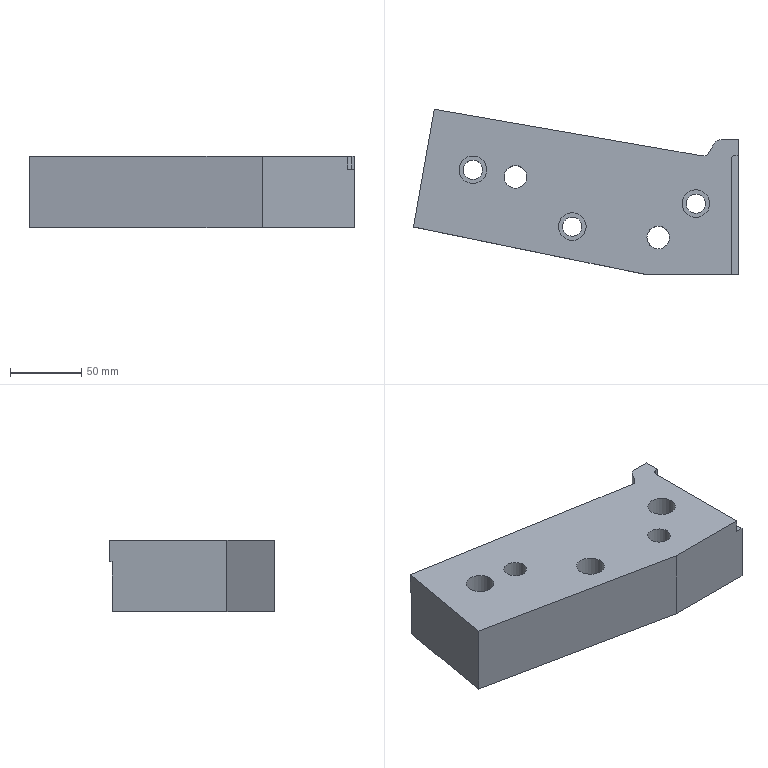Part | NX | features solid 2 | 1 solid | 29 faces | box 228.769 x 116.376 x 50 mm | volume 905067 mm3 | plane 16 | cylinder 9 | spline 4 | commonest cylinder face diameters 13.5 x3 19.5 x3 16 x2 6 x1
STEP:
#1=CARTESIAN_POINT('',(1123.262,283.786,0.));
#2=VERTEX_POINT('',#1);
#3=CARTESIAN_POINT('',(1133.012,283.786,0.));
#4=DIRECTION('',(0.,0.,-1.));
#5=DIRECTION('',(-1.,0.,0.));
#6=AXIS2_PLACEMENT_3D('',#3,#4,#5);
#7=CIRCLE('',#6,9.75);
#8=EDGE_CURVE('',#2,#2,#7,.F.);
#9=ORIENTED_EDGE('',*,*,#8,.F.);
#10=EDGE_LOOP('',(#9));
#11=FACE_BOUND('',#10,.T.);
#12=CARTESIAN_POINT('',(1053.262,323.786,0.));
#13=VERTEX_POINT('',#12);
#14=CARTESIAN_POINT('',(1063.012,323.786,0.));
#15=DIRECTION('',(0.,0.,-1.));
#16=DIRECTION('',(-1.,0.,0.));
#17=AXIS2_PLACEMENT_3D('',#14,#15,#16);
#18=CIRCLE('',#17,9.75);
#19=EDGE_CURVE('',#13,#13,#18,.F.);
#20=ORIENTED_EDGE('',*,*,#19,.F.);
#21=EDGE_LOOP('',(#20));
#22=FACE_BOUND('',#21,.T.);
#23=CARTESIAN_POINT('',(1210.25,300.,0.));
#24=VERTEX_POINT('',#23);
#25=CARTESIAN_POINT('',(1220.,300.,0.));
#26=DIRECTION('',(0.,0.,-1.));
#27=DIRECTION('',(-1.,0.,0.));
#28=AXIS2_PLACEMENT_3D('',#25,#26,#27);
#29=CIRCLE('',#28,9.75);
#30=EDGE_CURVE('',#24,#24,#29,.F.);
#31=ORIENTED_EDGE('',*,*,#30,.F.);
#32=EDGE_LOOP('',(#31));
#33=FACE_BOUND('',#32,.T.);
#34=CARTESIAN_POINT('',(1185.589,276.087,0.));
#35=VERTEX_POINT('',#34);
#36=CARTESIAN_POINT('',(1193.589,276.087,0.));
#37=DIRECTION('',(0.,0.,-1.));
#38=DIRECTION('',(-1.,0.,0.));
#39=AXIS2_PLACEMENT_3D('',#36,#37,#38);
#40=CIRCLE('',#39,8.);
#41=EDGE_CURVE('',#35,#35,#40,.F.);
#42=ORIENTED_EDGE('',*,*,#41,.F.);
#43=EDGE_LOOP('',(#42));
#44=FACE_BOUND('',#43,.T.);
#45=CARTESIAN_POINT('',(1021.231,283.553,0.));
#46=VERTEX_POINT('',#45);
#47=CARTESIAN_POINT('',(1035.834,366.376,0.));
#48=VERTEX_POINT('',#47);
#49=CARTESIAN_POINT('',(1025.414,307.279,0.));
#50=DIRECTION('',(0.1736,0.9848,0.));
#51=VECTOR('',#50,1000.);
#52=LINE('',#49,#51);
#53=EDGE_CURVE('',#46,#48,#52,.T.);
#54=ORIENTED_EDGE('',*,*,#53,.F.);
#55=CARTESIAN_POINT('',(1185.,250.,0.));
#56=VERTEX_POINT('',#55);
#57=CARTESIAN_POINT('',(1017.086,284.403,0.));
#58=DIRECTION('',(0.9797,-0.2007,0.));
#59=VECTOR('',#58,1000.);
#60=LINE('',#57,#59);
#61=EDGE_CURVE('',#46,#56,#60,.T.);
#62=ORIENTED_EDGE('',*,*,#61,.T.);
#63=CARTESIAN_POINT('',(1245.,250.,0.));
#64=VERTEX_POINT('',#63);
#65=CARTESIAN_POINT('',(1245.,250.,0.));
#66=DIRECTION('',(-1.,0.,0.));
#67=VECTOR('',#66,1000.);
#68=LINE('',#65,#67);
#69=EDGE_CURVE('',#56,#64,#68,.F.);
#70=ORIENTED_EDGE('',*,*,#69,.T.);
#71=CARTESIAN_POINT('',(1245.,331.,0.));
#72=VERTEX_POINT('',#71);
#73=CARTESIAN_POINT('',(1245.,307.899,0.));
#74=DIRECTION('',(0.,1.,0.));
#75=VECTOR('',#74,1000.);
#76=LINE('',#73,#75);
#77=EDGE_CURVE('',#64,#72,#76,.T.);
#78=ORIENTED_EDGE('',*,*,#77,.T.);
#79=CARTESIAN_POINT('',(1248.,334.,0.));
#80=VERTEX_POINT('',#79);
#81=CARTESIAN_POINT('',(1248.,331.,0.));
#82=DIRECTION('',(0.,0.,-1.));
#83=DIRECTION('',(-1.,0.,0.));
#84=AXIS2_PLACEMENT_3D('',#81,#82,#83);
#85=CIRCLE('',#84,3.);
#86=EDGE_CURVE('',#72,#80,#85,.T.);
#87=ORIENTED_EDGE('',*,*,#86,.T.);
#88=CARTESIAN_POINT('',(1250.,334.,0.));
#89=VERTEX_POINT('',#88);
#90=CARTESIAN_POINT('',(1021.9,334.,0.));
#91=DIRECTION('',(1.,0.,0.));
#92=VECTOR('',#91,1000.);
#93=LINE('',#90,#92);
#94=EDGE_CURVE('',#89,#80,#93,.F.);
#95=ORIENTED_EDGE('',*,*,#94,.F.);
#96=CARTESIAN_POINT('',(1250.,345.,0.));
#97=VERTEX_POINT('',#96);
#98=CARTESIAN_POINT('',(1250.,340.,0.));
#99=DIRECTION('',(0.,-1.,0.));
#100=VECTOR('',#99,1000.);
#101=LINE('',#98,#100);
#102=EDGE_CURVE('',#97,#89,#101,.T.);
#103=ORIENTED_EDGE('',*,*,#102,.F.);
#104=CARTESIAN_POINT('',(1237.889,345.,0.));
#105=VERTEX_POINT('',#104);
#106=CARTESIAN_POINT('',(1021.9,345.,0.));
#107=DIRECTION('',(-1.,0.,0.));
#108=VECTOR('',#107,1000.);
#109=LINE('',#106,#108);
#110=EDGE_CURVE('',#97,#105,#109,.T.);
#111=ORIENTED_EDGE('',*,*,#110,.T.);
#112=CARTESIAN_POINT('',(1231.463,339.803,0.));
#113=VERTEX_POINT('',#112);
#114=CARTESIAN_POINT('',(1231.463,339.803,0.));
#115=CARTESIAN_POINT('',(1232.171,341.078,0.));
#116=CARTESIAN_POINT('',(1233.286,342.988,0.));
#117=CARTESIAN_POINT('',(1235.696,344.739,0.));
#118=CARTESIAN_POINT('',(1237.155,345.,0.));
#119=CARTESIAN_POINT('',(1237.889,345.,0.));
#120=B_SPLINE_CURVE_WITH_KNOTS('',3,(#114,#115,#116,#117,#118,#119),.UNSPECIFIED.,.F.,.F.,(4,1,1,4),(0.05738,0.06181,0.06402,0.06624),.UNSPECIFIED.);
#121=EDGE_CURVE('',#113,#105,#120,.T.);
#122=ORIENTED_EDGE('',*,*,#121,.F.);
#123=CARTESIAN_POINT('',(1224.486,333.568,0.));
#124=VERTEX_POINT('',#123);
#125=CARTESIAN_POINT('',(1224.486,333.568,0.));
#126=CARTESIAN_POINT('',(1231.05,332.426,0.));
#127=CARTESIAN_POINT('',(1230.692,345.,0.));
#128=CARTESIAN_POINT('',(1237.854,345.,0.));
#129=B_SPLINE_CURVE_WITH_KNOTS('',3,(#125,#126,#127,#128),.UNSPECIFIED.,.F.,.F.,(4,4),(0.,1.),.PIECEWISE_BEZIER_KNOTS.);
#130=EDGE_CURVE('',#124,#113,#129,.T.);
#131=ORIENTED_EDGE('',*,*,#130,.F.);
#132=CARTESIAN_POINT('',(1187.5,340.,0.));
#133=VERTEX_POINT('',#132);
#134=CARTESIAN_POINT('',(1228.,332.956,0.));
#135=DIRECTION('',(-0.9852,0.1713,0.));
#136=VECTOR('',#135,1000.);
#137=LINE('',#134,#136);
#138=EDGE_CURVE('',#124,#133,#137,.T.);
#139=ORIENTED_EDGE('',*,*,#138,.T.);
#140=CARTESIAN_POINT('',(1323.576,316.335,0.));
#141=CARTESIAN_POINT('',(1303.952,319.748,0.));
#142=CARTESIAN_POINT('',(1284.328,323.16,0.));
#143=CARTESIAN_POINT('',(1264.704,326.573,0.));
#144=CARTESIAN_POINT('',(1233.889,331.932,0.));
#145=CARTESIAN_POINT('',(1172.258,342.651,0.));
#146=CARTESIAN_POINT('',(1095.22,356.049,0.));
#147=CARTESIAN_POINT('',(1033.589,366.767,0.));
#148=CARTESIAN_POINT('',(987.365,374.804,0.));
#149=CARTESIAN_POINT('',(948.847,381.509,0.));
#150=CARTESIAN_POINT('',(923.808,385.853,0.));
#151=CARTESIAN_POINT('',(914.109,387.486,0.));
#152=CARTESIAN_POINT('',(912.091,387.827,0.));
#153=CARTESIAN_POINT('',(911.971,387.848,0.));
#154=CARTESIAN_POINT('',(911.79,387.876,0.));
#155=CARTESIAN_POINT('',(911.394,387.917,0.));
#156=CARTESIAN_POINT('',(910.546,388.022,0.));
#157=CARTESIAN_POINT('',(908.847,388.221,0.));
#158=CARTESIAN_POINT('',(906.42,388.511,0.));
#159=CARTESIAN_POINT('',(903.994,388.799,0.));
#160=CARTESIAN_POINT('',(902.295,389.001,0.));
#161=CARTESIAN_POINT('',(901.446,389.101,0.));
#162=CARTESIAN_POINT('',(901.052,389.148,0.));
#163=CARTESIAN_POINT('',(900.87,389.17,0.));
#164=CARTESIAN_POINT('',(900.748,389.184,0.));
#165=CARTESIAN_POINT('',(899.68,389.239,0.));
#166=CARTESIAN_POINT('',(897.973,389.35,0.));
#167=CARTESIAN_POINT('',(896.023,389.486,0.));
#168=CARTESIAN_POINT('',(894.456,389.561,0.));
#169=CARTESIAN_POINT('',(892.989,389.903,0.));
#170=CARTESIAN_POINT('',(891.495,390.907,0.));
#171=CARTESIAN_POINT('',(890.458,392.378,0.));
#172=CARTESIAN_POINT('',(890.077,393.863,0.));
#173=CARTESIAN_POINT('',(889.825,397.101,0.));
#174=CARTESIAN_POINT('',(889.362,402.393,0.));
#175=CARTESIAN_POINT('',(888.928,407.354,0.));
#176=CARTESIAN_POINT('',(888.696,410.,0.));
#177=CARTESIAN_POINT('',(886.96,429.843,0.));
#178=CARTESIAN_POINT('',(885.224,449.685,0.));
#179=CARTESIAN_POINT('',(883.488,469.528,0.));
#180=B_SPLINE_CURVE_WITH_KNOTS('',3,(#140,#141,#142,#143,#144,#145,#146,#147,#148,#149,#150,#151,#152,#153,#154,#155,#156,#157,#158,#159,#160,#161,#162,#163,#164,#165,#166,#167,#168,#169,#170,#171,#172,#173,#174,#175,#176,#177,#178,#179),.UNSPECIFIED.,.F.,.F.,(4,3,1,1,1,1,1,1,1,1,1,1,1,1,1,1,1,1,1,1,1,1,1,1,1,1,1,1,1,1,1,1,3,4),(-0.15,0.,0.2355,0.4711,0.5889,0.7066,0.8244,0.8833,0.898,0.8985,0.8987,0.8989,0.8999,0.9017,0.9054,0.9127,0.9201,0.9238,0.9256,0.9265,0.9268,0.927,0.9275,0.9348,0.9399,0.9422,0.9466,0.9511,0.9555,0.96,0.9625,0.98,1.,1.15),.UNSPECIFIED.);
#181=EDGE_CURVE('',#133,#48,#180,.T.);
#182=ORIENTED_EDGE('',*,*,#181,.T.);
#183=EDGE_LOOP('',(#54,#62,#70,#78,#87,#95,#103,#111,#122,#131,#139,#182));
#184=FACE_BOUND('',#183,.T.);
#185=CARTESIAN_POINT('',(1085.012,318.786,0.));
#186=VERTEX_POINT('',#185);
#187=CARTESIAN_POINT('',(1093.012,318.786,0.));
#188=DIRECTION('',(0.,0.,-1.));
#189=DIRECTION('',(-1.,0.,0.));
#190=AXIS2_PLACEMENT_3D('',#187,#188,#189);
#191=CIRCLE('',#190,8.);
#192=EDGE_CURVE('',#186,#186,#191,.F.);
#193=ORIENTED_EDGE('',*,*,#192,.F.);
#194=EDGE_LOOP('',(#193));
#195=FACE_BOUND('',#194,.T.);
#196=CARTESIAN_POINT('',(1021.9,307.899,0.));
#197=DIRECTION('',(0.,0.,-1.));
#198=DIRECTION('',(1.,0.,0.));
#199=AXIS2_PLACEMENT_3D('',#196,#197,#198);
#200=PLANE('',#199);
#201=ADVANCED_FACE('',(#11,#22,#33,#44,#184,#195),#200,.F.);
#202=CARTESIAN_POINT('',(1126.262,283.786,-50.));
#203=VERTEX_POINT('',#202);
#204=CARTESIAN_POINT('',(1133.012,283.786,-50.));
#205=DIRECTION('',(0.,0.,-1.));
#206=DIRECTION('',(-1.,0.,0.));
#207=AXIS2_PLACEMENT_3D('',#204,#205,#206);
#208=CIRCLE('',#207,6.75);
#209=EDGE_CURVE('',#203,#203,#208,.F.);
#210=ORIENTED_EDGE('',*,*,#209,.T.);
#211=EDGE_LOOP('',(#210));
#212=FACE_BOUND('',#211,.T.);
#213=CARTESIAN_POINT('',(1056.262,323.786,-50.));
#214=VERTEX_POINT('',#213);
#215=CARTESIAN_POINT('',(1063.012,323.786,-50.));
#216=DIRECTION('',(0.,0.,-1.));
#217=DIRECTION('',(-1.,0.,0.));
#218=AXIS2_PLACEMENT_3D('',#215,#216,#217);
#219=CIRCLE('',#218,6.75);
#220=EDGE_CURVE('',#214,#214,#219,.F.);
#221=ORIENTED_EDGE('',*,*,#220,.T.);
#222=EDGE_LOOP('',(#221));
#223=FACE_BOUND('',#222,.T.);
#224=CARTESIAN_POINT('',(1213.25,300.,-50.));
#225=VERTEX_POINT('',#224);
#226=CARTESIAN_POINT('',(1220.,300.,-50.));
#227=DIRECTION('',(0.,0.,-1.));
#228=DIRECTION('',(-1.,0.,0.));
#229=AXIS2_PLACEMENT_3D('',#226,#227,#228);
#230=CIRCLE('',#229,6.75);
#231=EDGE_CURVE('',#225,#225,#230,.F.);
#232=ORIENTED_EDGE('',*,*,#231,.T.);
#233=EDGE_LOOP('',(#232));
#234=FACE_BOUND('',#233,.T.);
#235=CARTESIAN_POINT('',(1185.589,276.087,-50.));
#236=VERTEX_POINT('',#235);
#237=CARTESIAN_POINT('',(1193.589,276.087,-50.));
#238=DIRECTION('',(0.,0.,-1.));
#239=DIRECTION('',(-1.,0.,0.));
#240=AXIS2_PLACEMENT_3D('',#237,#238,#239);
#241=CIRCLE('',#240,8.);
#242=EDGE_CURVE('',#236,#236,#241,.F.);
#243=ORIENTED_EDGE('',*,*,#242,.T.);
#244=EDGE_LOOP('',(#243));
#245=FACE_BOUND('',#244,.T.);
#246=CARTESIAN_POINT('',(1021.231,283.553,-50.));
#247=VERTEX_POINT('',#246);
#248=CARTESIAN_POINT('',(1185.,250.,-50.));
#249=VERTEX_POINT('',#248);
#250=CARTESIAN_POINT('',(1017.086,284.403,-50.));
#251=DIRECTION('',(0.9797,-0.2007,0.));
#252=VECTOR('',#251,1000.);
#253=LINE('',#250,#252);
#254=EDGE_CURVE('',#247,#249,#253,.T.);
#255=ORIENTED_EDGE('',*,*,#254,.F.);
#256=CARTESIAN_POINT('',(1035.487,364.407,-50.));
#257=VERTEX_POINT('',#256);
#258=CARTESIAN_POINT('',(1025.414,307.279,-50.));
#259=DIRECTION('',(0.1736,0.9848,0.));
#260=VECTOR('',#259,1000.);
#261=LINE('',#258,#260);
#262=EDGE_CURVE('',#247,#257,#261,.T.);
#263=ORIENTED_EDGE('',*,*,#262,.T.);
#264=CARTESIAN_POINT('',(1224.144,331.597,-50.));
#265=VERTEX_POINT('',#264);
#266=CARTESIAN_POINT('',(1035.487,364.408,-50.));
#267=CARTESIAN_POINT('',(1098.372,353.464,-50.));
#268=CARTESIAN_POINT('',(1161.256,342.523,-50.));
#269=CARTESIAN_POINT('',(1224.143,331.595,-50.));
#270=B_SPLINE_CURVE_WITH_KNOTS('',3,(#266,#267,#268,#269),.UNSPECIFIED.,.F.,.F.,(4,4),(0.4726,0.9521),.UNSPECIFIED.);
#271=EDGE_CURVE('',#265,#257,#270,.F.);
#272=ORIENTED_EDGE('',*,*,#271,.F.);
#273=CARTESIAN_POINT('',(1232.756,337.998,-50.));
#274=VERTEX_POINT('',#273);
#275=CARTESIAN_POINT('',(1224.143,331.597,-50.));
#276=CARTESIAN_POINT('',(1225.228,331.409,-50.));
#277=CARTESIAN_POINT('',(1226.743,331.5,-50.));
#278=CARTESIAN_POINT('',(1228.346,332.296,-50.));
#279=CARTESIAN_POINT('',(1229.18,332.908,-50.));
#280=CARTESIAN_POINT('',(1229.861,333.556,-50.));
#281=CARTESIAN_POINT('',(1230.2,333.942,-50.));
#282=CARTESIAN_POINT('',(1230.629,334.473,-50.));
#283=CARTESIAN_POINT('',(1230.974,334.958,-50.));
#284=CARTESIAN_POINT('',(1231.239,335.355,-50.));
#285=CARTESIAN_POINT('',(1231.48,335.737,-50.));
#286=CARTESIAN_POINT('',(1231.56,335.871,-50.));
#287=CARTESIAN_POINT('',(1231.745,336.182,-50.));
#288=CARTESIAN_POINT('',(1232.087,336.777,-50.));
#289=CARTESIAN_POINT('',(1232.468,337.468,-50.));
#290=CARTESIAN_POINT('',(1232.756,337.998,-50.));
#291=B_SPLINE_CURVE_WITH_KNOTS('',3,(#275,#276,#277,#278,#279,#280,#281,#282,#283,#284,#285,#286,#287,#288,#289,#290),.UNSPECIFIED.,.F.,.F.,(4,1,1,1,1,1,1,1,1,1,1,1,1,4),(0.,0.25,0.375,0.4375,0.5,0.5625,0.625,0.6875,0.7188,0.75,0.7812,0.8125,0.875,1.),.UNSPECIFIED.);
#292=EDGE_CURVE('',#265,#274,#291,.T.);
#293=ORIENTED_EDGE('',*,*,#292,.T.);
#294=CARTESIAN_POINT('',(1237.854,343.,-50.));
#295=VERTEX_POINT('',#294);
#296=CARTESIAN_POINT('',(1232.755,337.999,-50.));
#297=CARTESIAN_POINT('',(1233.177,338.771,-50.));
#298=CARTESIAN_POINT('',(1233.575,339.487,-50.));
#299=CARTESIAN_POINT('',(1233.966,340.122,-50.));
#300=CARTESIAN_POINT('',(1234.076,340.296,-50.));
#301=CARTESIAN_POINT('',(1234.264,340.582,-50.));
#302=CARTESIAN_POINT('',(1234.523,340.953,-50.));
#303=CARTESIAN_POINT('',(1234.918,341.464,-50.));
#304=CARTESIAN_POINT('',(1235.316,341.895,-50.));
#305=CARTESIAN_POINT('',(1235.691,342.232,-50.));
#306=CARTESIAN_POINT('',(1236.515,342.818,-50.));
#307=CARTESIAN_POINT('',(1237.221,343.,-50.));
#308=CARTESIAN_POINT('',(1237.854,343.,-50.));
#309=B_SPLINE_CURVE_WITH_KNOTS('',3,(#296,#297,#298,#299,#300,#301,#302,#303,#304,#305,#306,#307,#308),.UNSPECIFIED.,.F.,.F.,(4,1,1,1,1,1,1,1,1,1,4),(0.613,0.7098,0.734,0.7461,0.7582,0.7823,0.8065,0.8549,0.8791,0.9033,1.),.UNSPECIFIED.);
#310=EDGE_CURVE('',#274,#295,#309,.T.);
#311=ORIENTED_EDGE('',*,*,#310,.T.);
#312=CARTESIAN_POINT('',(1250.,343.,-50.));
#313=VERTEX_POINT('',#312);
#314=CARTESIAN_POINT('',(1021.9,343.,-50.));
#315=DIRECTION('',(-1.,0.,0.));
#316=VECTOR('',#315,1000.);
#317=LINE('',#314,#316);
#318=EDGE_CURVE('',#313,#295,#317,.T.);
#319=ORIENTED_EDGE('',*,*,#318,.F.);
#320=CARTESIAN_POINT('',(1250.,250.,-50.));
#321=VERTEX_POINT('',#320);
#322=CARTESIAN_POINT('',(1250.,307.899,-50.));
#323=DIRECTION('',(0.,1.,0.));
#324=VECTOR('',#323,1000.);
#325=LINE('',#322,#324);
#326=EDGE_CURVE('',#321,#313,#325,.T.);
#327=ORIENTED_EDGE('',*,*,#326,.F.);
#328=CARTESIAN_POINT('',(1245.,250.,-50.));
#329=DIRECTION('',(-1.,0.,0.));
#330=VECTOR('',#329,1000.);
#331=LINE('',#328,#330);
#332=EDGE_CURVE('',#321,#249,#331,.T.);
#333=ORIENTED_EDGE('',*,*,#332,.T.);
#334=EDGE_LOOP('',(#255,#263,#272,#293,#311,#319,#327,#333));
#335=FACE_BOUND('',#334,.T.);
#336=CARTESIAN_POINT('',(1085.012,318.786,-50.));
#337=VERTEX_POINT('',#336);
#338=CARTESIAN_POINT('',(1093.012,318.786,-50.));
#339=DIRECTION('',(0.,0.,-1.));
#340=DIRECTION('',(-1.,0.,0.));
#341=AXIS2_PLACEMENT_3D('',#338,#339,#340);
#342=CIRCLE('',#341,8.);
#343=EDGE_CURVE('',#337,#337,#342,.F.);
#344=ORIENTED_EDGE('',*,*,#343,.T.);
#345=EDGE_LOOP('',(#344));
#346=FACE_BOUND('',#345,.T.);
#347=CARTESIAN_POINT('',(1021.9,307.899,-50.));
#348=DIRECTION('',(0.,0.,-1.));
#349=DIRECTION('',(1.,0.,0.));
#350=AXIS2_PLACEMENT_3D('',#347,#348,#349);
#351=PLANE('',#350);
#352=ADVANCED_FACE('',(#212,#223,#234,#245,#335,#346),#351,.T.);
#353=CARTESIAN_POINT('',(1035.487,364.406,-15.));
#354=VERTEX_POINT('',#353);
#355=CARTESIAN_POINT('',(1035.487,364.406,-32.5));
#356=DIRECTION('',(0.,0.,1.));
#357=VECTOR('',#356,1000.);
#358=LINE('',#355,#357);
#359=EDGE_CURVE('',#354,#257,#358,.F.);
#360=ORIENTED_EDGE('',*,*,#359,.F.);
#361=CARTESIAN_POINT('',(1224.143,331.597,-15.));
#362=VERTEX_POINT('',#361);
#363=CARTESIAN_POINT('',(1035.487,364.406,-15.));
#364=CARTESIAN_POINT('',(1098.373,353.471,-15.));
#365=CARTESIAN_POINT('',(1161.258,342.534,-15.));
#366=CARTESIAN_POINT('',(1224.143,331.597,-15.));
#367=B_SPLINE_CURVE_WITH_KNOTS('',3,(#363,#364,#365,#366),.UNSPECIFIED.,.F.,.F.,(4,4),(0.8083,0.9998),.UNSPECIFIED.);
#368=EDGE_CURVE('',#362,#354,#367,.F.);
#369=ORIENTED_EDGE('',*,*,#368,.F.);
#370=CARTESIAN_POINT('',(1224.143,331.597,-15.));
#371=DIRECTION('',(0.,0.,-1.));
#372=VECTOR('',#371,1000.);
#373=LINE('',#370,#372);
#374=EDGE_CURVE('',#362,#265,#373,.T.);
#375=ORIENTED_EDGE('',*,*,#374,.T.);
#376=ORIENTED_EDGE('',*,*,#271,.T.);
#377=EDGE_LOOP('',(#360,#369,#375,#376));
#378=FACE_BOUND('',#377,.T.);
#379=CARTESIAN_POINT('',(1225.276,331.4,-50.));
#380=CARTESIAN_POINT('',(1225.276,331.4,-15.));
#381=CARTESIAN_POINT('',(1162.013,342.402,-50.));
#382=CARTESIAN_POINT('',(1162.013,342.402,-15.));
#383=CARTESIAN_POINT('',(1098.75,353.405,-50.));
#384=CARTESIAN_POINT('',(1098.75,353.405,-15.));
#385=CARTESIAN_POINT('',(1035.487,364.406,-50.));
#386=CARTESIAN_POINT('',(1035.487,364.406,-15.));
#387=B_SPLINE_SURFACE_WITH_KNOTS('',3,1,((#379,#380),(#381,#382),(#383,#384),(#385,#386)),.SURF_OF_LINEAR_EXTRUSION.,.F.,.F.,.F.,(4,4),(2,2),(0.09649,0.5817),(0.,1.),.PIECEWISE_BEZIER_KNOTS.);
#388=ADVANCED_FACE('',(#378),#387,.T.);
#389=CARTESIAN_POINT('',(1035.834,366.376,-15.));
#390=VERTEX_POINT('',#389);
#391=CARTESIAN_POINT('',(1035.834,366.376,-7.5));
#392=DIRECTION('',(0.,0.,1.));
#393=VECTOR('',#392,1000.);
#394=LINE('',#391,#393);
#395=EDGE_CURVE('',#48,#390,#394,.F.);
#396=ORIENTED_EDGE('',*,*,#395,.F.);
#397=ORIENTED_EDGE('',*,*,#181,.F.);
#398=CARTESIAN_POINT('',(1187.5,340.,-15.));
#399=VERTEX_POINT('',#398);
#400=CARTESIAN_POINT('',(1187.5,340.,0.));
#401=DIRECTION('',(0.,0.,-1.));
#402=VECTOR('',#401,1000.);
#403=LINE('',#400,#402);
#404=EDGE_CURVE('',#399,#133,#403,.F.);
#405=ORIENTED_EDGE('',*,*,#404,.F.);
#406=CARTESIAN_POINT('',(1045.24,364.741,-15.));
#407=VERTEX_POINT('',#406);
#408=CARTESIAN_POINT('',(1187.5,340.,-15.));
#409=CARTESIAN_POINT('',(1140.08,348.247,-15.));
#410=CARTESIAN_POINT('',(1092.66,356.494,-15.));
#411=CARTESIAN_POINT('',(1045.24,364.741,-15.));
#412=B_SPLINE_CURVE_WITH_KNOTS('',3,(#408,#409,#410,#411),.UNSPECIFIED.,.F.,.F.,(4,4),(0.05836,0.2028),.UNSPECIFIED.);
#413=EDGE_CURVE('',#399,#407,#412,.T.);
#414=ORIENTED_EDGE('',*,*,#413,.T.);
#415=CARTESIAN_POINT('',(1035.834,366.376,-15.));
#416=CARTESIAN_POINT('',(1038.848,365.852,-15.));
#417=CARTESIAN_POINT('',(1041.983,365.307,-15.));
#418=CARTESIAN_POINT('',(1045.24,364.741,-15.));
#419=B_SPLINE_CURVE_WITH_KNOTS('',3,(#415,#416,#417,#418),.UNSPECIFIED.,.F.,.F.,(4,4),(0.9049,1.),.UNSPECIFIED.);
#420=EDGE_CURVE('',#407,#390,#419,.F.);
#421=ORIENTED_EDGE('',*,*,#420,.T.);
#422=EDGE_LOOP('',(#396,#397,#405,#414,#421));
#423=FACE_BOUND('',#422,.T.);
#424=CARTESIAN_POINT('',(1187.5,340.,-15.));
#425=CARTESIAN_POINT('',(1187.5,340.,0.));
#426=CARTESIAN_POINT('',(1136.945,348.792,-15.));
#427=CARTESIAN_POINT('',(1136.945,348.792,0.));
#428=CARTESIAN_POINT('',(1086.39,357.585,-15.));
#429=CARTESIAN_POINT('',(1086.39,357.585,0.));
#430=CARTESIAN_POINT('',(1035.834,366.376,-15.));
#431=CARTESIAN_POINT('',(1035.834,366.376,0.));
#432=B_SPLINE_SURFACE_WITH_KNOTS('',3,1,((#424,#425),(#426,#427),(#428,#429),(#430,#431)),.SURF_OF_LINEAR_EXTRUSION.,.F.,.F.,.F.,(4,4),(2,2),(0.1967,0.5831),(0.,1.),.PIECEWISE_BEZIER_KNOTS.);
#433=ADVANCED_FACE('',(#423),#432,.T.);
#434=CARTESIAN_POINT('',(1022.389,290.122,-15.));
#435=DIRECTION('',(0.1736,0.9848,0.));
#436=VECTOR('',#435,1000.);
#437=LINE('',#434,#436);
#438=EDGE_CURVE('',#390,#354,#437,.F.);
#439=ORIENTED_EDGE('',*,*,#438,.F.);
#440=ORIENTED_EDGE('',*,*,#420,.F.);
#441=ORIENTED_EDGE('',*,*,#413,.F.);
#442=CARTESIAN_POINT('',(1224.486,333.568,-15.));
#443=VERTEX_POINT('',#442);
#444=CARTESIAN_POINT('',(1258.358,327.677,-15.));
#445=DIRECTION('',(0.9852,-0.1713,0.));
#446=VECTOR('',#445,1000.);
#447=LINE('',#444,#446);
#448=EDGE_CURVE('',#443,#399,#447,.F.);
#449=ORIENTED_EDGE('',*,*,#448,.F.);
#450=CARTESIAN_POINT('',(1237.854,345.,-15.));
#451=VERTEX_POINT('',#450);
#452=CARTESIAN_POINT('',(1224.486,333.568,-15.));
#453=CARTESIAN_POINT('',(1231.05,332.426,-15.));
#454=CARTESIAN_POINT('',(1230.692,345.,-15.));
#455=CARTESIAN_POINT('',(1237.854,345.,-15.));
#456=B_SPLINE_CURVE_WITH_KNOTS('',3,(#452,#453,#454,#455),.UNSPECIFIED.,.F.,.F.,(4,4),(0.,1.),.PIECEWISE_BEZIER_KNOTS.);
#457=EDGE_CURVE('',#443,#451,#456,.T.);
#458=ORIENTED_EDGE('',*,*,#457,.T.);
#459=CARTESIAN_POINT('',(1250.,345.,-15.));
#460=VERTEX_POINT('',#459);
#461=CARTESIAN_POINT('',(1250.,345.,-15.));
#462=DIRECTION('',(-1.,0.,0.));
#463=VECTOR('',#462,1000.);
#464=LINE('',#461,#463);
#465=EDGE_CURVE('',#460,#451,#464,.T.);
#466=ORIENTED_EDGE('',*,*,#465,.F.);
#467=CARTESIAN_POINT('',(1250.,343.,-15.));
#468=VERTEX_POINT('',#467);
#469=CARTESIAN_POINT('',(1250.,390.,-15.));
#470=DIRECTION('',(0.,1.,0.));
#471=VECTOR('',#470,1000.);
#472=LINE('',#469,#471);
#473=EDGE_CURVE('',#460,#468,#472,.F.);
#474=ORIENTED_EDGE('',*,*,#473,.T.);
#475=CARTESIAN_POINT('',(1237.854,343.,-15.));
#476=VERTEX_POINT('',#475);
#477=CARTESIAN_POINT('',(1250.,343.,-15.));
#478=DIRECTION('',(-1.,0.,0.));
#479=VECTOR('',#478,1000.);
#480=LINE('',#477,#479);
#481=EDGE_CURVE('',#468,#476,#480,.T.);
#482=ORIENTED_EDGE('',*,*,#481,.T.);
#483=CARTESIAN_POINT('',(1233.89,340.,-15.));
#484=VERTEX_POINT('',#483);
#485=CARTESIAN_POINT('',(1233.89,340.,-15.));
#486=CARTESIAN_POINT('',(1234.534,341.043,-15.));
#487=CARTESIAN_POINT('',(1235.689,342.507,-15.));
#488=CARTESIAN_POINT('',(1237.072,343.,-15.));
#489=CARTESIAN_POINT('',(1237.854,343.,-15.));
#490=B_SPLINE_CURVE_WITH_KNOTS('',3,(#485,#486,#487,#488,#489),.UNSPECIFIED.,.F.,.F.,(4,1,4),(0.,0.5,1.),.UNSPECIFIED.);
#491=EDGE_CURVE('',#484,#476,#490,.T.);
#492=ORIENTED_EDGE('',*,*,#491,.F.);
#493=CARTESIAN_POINT('',(1232.756,337.998,-15.));
#494=VERTEX_POINT('',#493);
#495=CARTESIAN_POINT('',(1233.89,340.,-15.));
#496=CARTESIAN_POINT('',(1233.512,339.333,-15.));
#497=CARTESIAN_POINT('',(1233.134,338.666,-15.));
#498=CARTESIAN_POINT('',(1232.756,337.998,-15.));
#499=B_SPLINE_CURVE_WITH_KNOTS('',3,(#495,#496,#497,#498),.UNSPECIFIED.,.F.,.F.,(4,4),(0.,1.),.UNSPECIFIED.);
#500=EDGE_CURVE('',#494,#484,#499,.F.);
#501=ORIENTED_EDGE('',*,*,#500,.F.);
#502=CARTESIAN_POINT('',(1224.143,331.597,-15.));
#503=CARTESIAN_POINT('',(1225.228,331.409,-15.));
#504=CARTESIAN_POINT('',(1226.744,331.502,-15.));
#505=CARTESIAN_POINT('',(1228.342,332.293,-15.));
#506=CARTESIAN_POINT('',(1229.183,332.912,-15.));
#507=CARTESIAN_POINT('',(1229.842,333.536,-15.));
#508=CARTESIAN_POINT('',(1230.19,333.929,-15.));
#509=CARTESIAN_POINT('',(1230.626,334.469,-15.));
#510=CARTESIAN_POINT('',(1231.022,335.02,-15.));
#511=CARTESIAN_POINT('',(1231.411,335.625,-15.));
#512=CARTESIAN_POINT('',(1231.549,335.853,-15.));
#513=CARTESIAN_POINT('',(1231.738,336.169,-15.));
#514=CARTESIAN_POINT('',(1232.088,336.777,-15.));
#515=CARTESIAN_POINT('',(1232.494,337.517,-15.));
#516=CARTESIAN_POINT('',(1232.756,337.998,-15.));
#517=B_SPLINE_CURVE_WITH_KNOTS('',3,(#502,#503,#504,#505,#506,#507,#508,#509,#510,#511,#512,#513,#514,#515,#516),.UNSPECIFIED.,.F.,.F.,(4,1,1,1,1,1,1,1,1,1,1,1,4),(0.,0.126,0.189,0.2206,0.2521,0.2836,0.3151,0.3466,0.3781,0.3939,0.4096,0.4411,0.5041),.UNSPECIFIED.);
#518=EDGE_CURVE('',#362,#494,#517,.T.);
#519=ORIENTED_EDGE('',*,*,#518,.F.);
#520=ORIENTED_EDGE('',*,*,#368,.T.);
#521=EDGE_LOOP('',(#439,#440,#441,#449,#458,#466,#474,#482,#492,#501,#519,#520));
#522=FACE_BOUND('',#521,.T.);
#523=CARTESIAN_POINT('',(1245.,250.87,-15.));
#524=DIRECTION('',(0.,0.,-1.));
#525=DIRECTION('',(0.,1.,0.));
#526=AXIS2_PLACEMENT_3D('',#523,#524,#525);
#527=PLANE('',#526);
#528=ADVANCED_FACE('',(#522),#527,.T.);
#529=CARTESIAN_POINT('',(1021.231,283.553,-50.));
#530=DIRECTION('',(0.,0.,1.));
#531=VECTOR('',#530,1000.);
#532=LINE('',#529,#531);
#533=EDGE_CURVE('',#247,#46,#532,.T.);
#534=ORIENTED_EDGE('',*,*,#533,.F.);
#535=ORIENTED_EDGE('',*,*,#254,.T.);
#536=CARTESIAN_POINT('',(1185.,250.,0.));
#537=DIRECTION('',(0.,0.,-1.));
#538=VECTOR('',#537,1000.);
#539=LINE('',#536,#538);
#540=EDGE_CURVE('',#56,#249,#539,.T.);
#541=ORIENTED_EDGE('',*,*,#540,.F.);
#542=ORIENTED_EDGE('',*,*,#61,.F.);
#543=EDGE_LOOP('',(#534,#535,#541,#542));
#544=FACE_BOUND('',#543,.T.);
#545=CARTESIAN_POINT('',(1185.,250.,-50.));
#546=DIRECTION('',(0.2007,0.9797,0.));
#547=DIRECTION('',(-0.9797,0.2007,0.));
#548=AXIS2_PLACEMENT_3D('',#545,#546,#547);
#549=PLANE('',#548);
#550=ADVANCED_FACE('',(#544),#549,.F.);
#551=ORIENTED_EDGE('',*,*,#102,.T.);
#552=CARTESIAN_POINT('',(1250.,334.,-9.));
#553=VERTEX_POINT('',#552);
#554=CARTESIAN_POINT('',(1250.,334.,-50.));
#555=DIRECTION('',(0.,0.,-1.));
#556=VECTOR('',#555,1000.);
#557=LINE('',#554,#556);
#558=EDGE_CURVE('',#553,#89,#557,.F.);
#559=ORIENTED_EDGE('',*,*,#558,.F.);
#560=CARTESIAN_POINT('',(1250.,250.,-9.));
#561=VERTEX_POINT('',#560);
#562=CARTESIAN_POINT('',(1250.,390.,-9.));
#563=DIRECTION('',(0.,-1.,0.));
#564=VECTOR('',#563,1000.);
#565=LINE('',#562,#564);
#566=EDGE_CURVE('',#561,#553,#565,.F.);
#567=ORIENTED_EDGE('',*,*,#566,.F.);
#568=CARTESIAN_POINT('',(1250.,250.,0.));
#569=DIRECTION('',(0.,0.,1.));
#570=VECTOR('',#569,1000.);
#571=LINE('',#568,#570);
#572=EDGE_CURVE('',#321,#561,#571,.T.);
#573=ORIENTED_EDGE('',*,*,#572,.F.);
#574=ORIENTED_EDGE('',*,*,#326,.T.);
#575=CARTESIAN_POINT('',(1250.,343.,-50.));
#576=DIRECTION('',(0.,0.,1.));
#577=VECTOR('',#576,1000.);
#578=LINE('',#575,#577);
#579=EDGE_CURVE('',#468,#313,#578,.F.);
#580=ORIENTED_EDGE('',*,*,#579,.F.);
#581=ORIENTED_EDGE('',*,*,#473,.F.);
#582=CARTESIAN_POINT('',(1250.,345.,-50.));
#583=DIRECTION('',(0.,0.,1.));
#584=VECTOR('',#583,1000.);
#585=LINE('',#582,#584);
#586=EDGE_CURVE('',#97,#460,#585,.F.);
#587=ORIENTED_EDGE('',*,*,#586,.F.);
#588=EDGE_LOOP('',(#551,#559,#567,#573,#574,#580,#581,#587));
#589=FACE_BOUND('',#588,.T.);
#590=CARTESIAN_POINT('',(1250.,390.,-50.));
#591=DIRECTION('',(-1.,0.,0.));
#592=DIRECTION('',(0.,0.,1.));
#593=AXIS2_PLACEMENT_3D('',#590,#591,#592);
#594=PLANE('',#593);
#595=ADVANCED_FACE('',(#589),#594,.F.);
#596=CARTESIAN_POINT('',(1245.,250.,-9.));
#597=VERTEX_POINT('',#596);
#598=CARTESIAN_POINT('',(1185.,250.,-9.));
#599=DIRECTION('',(-1.,0.,0.));
#600=VECTOR('',#599,1000.);
#601=LINE('',#598,#600);
#602=EDGE_CURVE('',#597,#561,#601,.F.);
#603=ORIENTED_EDGE('',*,*,#602,.F.);
#604=CARTESIAN_POINT('',(1245.,250.,0.));
#605=DIRECTION('',(0.,0.,1.));
#606=VECTOR('',#605,1000.);
#607=LINE('',#604,#606);
#608=EDGE_CURVE('',#597,#64,#607,.T.);
#609=ORIENTED_EDGE('',*,*,#608,.T.);
#610=ORIENTED_EDGE('',*,*,#69,.F.);
#611=ORIENTED_EDGE('',*,*,#540,.T.);
#612=ORIENTED_EDGE('',*,*,#332,.F.);
#613=ORIENTED_EDGE('',*,*,#572,.T.);
#614=EDGE_LOOP('',(#603,#609,#610,#611,#612,#613));
#615=FACE_BOUND('',#614,.T.);
#616=CARTESIAN_POINT('',(1185.,250.,0.));
#617=DIRECTION('',(0.,1.,0.));
#618=DIRECTION('',(0.,0.,1.));
#619=AXIS2_PLACEMENT_3D('',#616,#617,#618);
#620=PLANE('',#619);
#621=ADVANCED_FACE('',(#615),#620,.F.);
#622=CARTESIAN_POINT('',(1229.75,300.,-25.));
#623=VERTEX_POINT('',#622);
#624=CARTESIAN_POINT('',(1220.,300.,-25.));
#625=DIRECTION('',(0.,0.,1.));
#626=DIRECTION('',(1.,0.,0.));
#627=AXIS2_PLACEMENT_3D('',#624,#625,#626);
#628=CIRCLE('',#627,9.75);
#629=EDGE_CURVE('',#623,#623,#628,.T.);
#630=ORIENTED_EDGE('',*,*,#629,.T.);
#631=EDGE_LOOP('',(#630));
#632=FACE_BOUND('',#631,.T.);
#633=CARTESIAN_POINT('',(1226.75,300.,-25.));
#634=VERTEX_POINT('',#633);
#635=CARTESIAN_POINT('',(1220.,300.,-25.));
#636=DIRECTION('',(0.,0.,1.));
#637=DIRECTION('',(1.,0.,0.));
#638=AXIS2_PLACEMENT_3D('',#635,#636,#637);
#639=CIRCLE('',#638,6.75);
#640=EDGE_CURVE('',#634,#634,#639,.F.);
#641=ORIENTED_EDGE('',*,*,#640,.T.);
#642=EDGE_LOOP('',(#641));
#643=FACE_BOUND('',#642,.T.);
#644=CARTESIAN_POINT('',(1220.,300.,-25.));
#645=DIRECTION('',(0.,0.,1.));
#646=DIRECTION('',(1.,0.,0.));
#647=AXIS2_PLACEMENT_3D('',#644,#645,#646);
#648=PLANE('',#647);
#649=ADVANCED_FACE('',(#632,#643),#648,.T.);
#650=CARTESIAN_POINT('',(1072.762,323.786,-25.));
#651=VERTEX_POINT('',#650);
#652=CARTESIAN_POINT('',(1063.012,323.786,-25.));
#653=DIRECTION('',(0.,0.,1.));
#654=DIRECTION('',(1.,0.,0.));
#655=AXIS2_PLACEMENT_3D('',#652,#653,#654);
#656=CIRCLE('',#655,9.75);
#657=EDGE_CURVE('',#651,#651,#656,.T.);
#658=ORIENTED_EDGE('',*,*,#657,.T.);
#659=EDGE_LOOP('',(#658));
#660=FACE_BOUND('',#659,.T.);
#661=CARTESIAN_POINT('',(1069.762,323.786,-25.));
#662=VERTEX_POINT('',#661);
#663=CARTESIAN_POINT('',(1063.012,323.786,-25.));
#664=DIRECTION('',(0.,0.,1.));
#665=DIRECTION('',(1.,0.,0.));
#666=AXIS2_PLACEMENT_3D('',#663,#664,#665);
#667=CIRCLE('',#666,6.75);
#668=EDGE_CURVE('',#662,#662,#667,.F.);
#669=ORIENTED_EDGE('',*,*,#668,.T.);
#670=EDGE_LOOP('',(#669));
#671=FACE_BOUND('',#670,.T.);
#672=CARTESIAN_POINT('',(1063.012,323.786,-25.));
#673=DIRECTION('',(0.,0.,1.));
#674=DIRECTION('',(1.,0.,0.));
#675=AXIS2_PLACEMENT_3D('',#672,#673,#674);
#676=PLANE('',#675);
#677=ADVANCED_FACE('',(#660,#671),#676,.T.);
#678=ORIENTED_EDGE('',*,*,#657,.F.);
#679=EDGE_LOOP('',(#678));
#680=FACE_BOUND('',#679,.T.);
#681=ORIENTED_EDGE('',*,*,#19,.T.);
#682=EDGE_LOOP('',(#681));
#683=FACE_BOUND('',#682,.T.);
#684=CARTESIAN_POINT('',(1063.012,323.786,75.));
#685=DIRECTION('',(0.,0.,-1.));
#686=DIRECTION('',(-1.,0.,0.));
#687=AXIS2_PLACEMENT_3D('',#684,#685,#686);
#688=CYLINDRICAL_SURFACE('',#687,9.75);
#689=ADVANCED_FACE('',(#680,#683),#688,.F.);
#690=ORIENTED_EDGE('',*,*,#629,.F.);
#691=EDGE_LOOP('',(#690));
#692=FACE_BOUND('',#691,.T.);
#693=ORIENTED_EDGE('',*,*,#30,.T.);
#694=EDGE_LOOP('',(#693));
#695=FACE_BOUND('',#694,.T.);
#696=CARTESIAN_POINT('',(1220.,300.,75.));
#697=DIRECTION('',(0.,0.,-1.));
#698=DIRECTION('',(-1.,0.,0.));
#699=AXIS2_PLACEMENT_3D('',#696,#697,#698);
#700=CYLINDRICAL_SURFACE('',#699,9.75);
#701=ADVANCED_FACE('',(#692,#695),#700,.F.);
#702=ORIENTED_EDGE('',*,*,#220,.F.);
#703=EDGE_LOOP('',(#702));
#704=FACE_BOUND('',#703,.T.);
#705=ORIENTED_EDGE('',*,*,#668,.F.);
#706=EDGE_LOOP('',(#705));
#707=FACE_BOUND('',#706,.T.);
#708=CARTESIAN_POINT('',(1063.012,323.786,75.));
#709=DIRECTION('',(0.,0.,-1.));
#710=DIRECTION('',(-1.,0.,0.));
#711=AXIS2_PLACEMENT_3D('',#708,#709,#710);
#712=CYLINDRICAL_SURFACE('',#711,6.75);
#713=ADVANCED_FACE('',(#704,#707),#712,.F.);
#714=ORIENTED_EDGE('',*,*,#231,.F.);
#715=EDGE_LOOP('',(#714));
#716=FACE_BOUND('',#715,.T.);
#717=ORIENTED_EDGE('',*,*,#640,.F.);
#718=EDGE_LOOP('',(#717));
#719=FACE_BOUND('',#718,.T.);
#720=CARTESIAN_POINT('',(1220.,300.,75.));
#721=DIRECTION('',(0.,0.,-1.));
#722=DIRECTION('',(-1.,0.,0.));
#723=AXIS2_PLACEMENT_3D('',#720,#721,#722);
#724=CYLINDRICAL_SURFACE('',#723,6.75);
#725=ADVANCED_FACE('',(#716,#719),#724,.F.);
#726=ORIENTED_EDGE('',*,*,#242,.F.);
#727=EDGE_LOOP('',(#726));
#728=FACE_BOUND('',#727,.T.);
#729=ORIENTED_EDGE('',*,*,#41,.T.);
#730=EDGE_LOOP('',(#729));
#731=FACE_BOUND('',#730,.T.);
#732=CARTESIAN_POINT('',(1193.589,276.087,50.));
#733=DIRECTION('',(0.,0.,-1.));
#734=DIRECTION('',(-1.,0.,0.));
#735=AXIS2_PLACEMENT_3D('',#732,#733,#734);
#736=CYLINDRICAL_SURFACE('',#735,8.);
#737=ADVANCED_FACE('',(#728,#731),#736,.F.);
#738=CARTESIAN_POINT('',(1248.,334.,-9.));
#739=VERTEX_POINT('',#738);
#740=CARTESIAN_POINT('',(1250.,334.,-9.));
#741=DIRECTION('',(-1.,0.,0.));
#742=VECTOR('',#741,1000.);
#743=LINE('',#740,#742);
#744=EDGE_CURVE('',#553,#739,#743,.T.);
#745=ORIENTED_EDGE('',*,*,#744,.T.);
#746=CARTESIAN_POINT('',(1245.,331.,-9.));
#747=VERTEX_POINT('',#746);
#748=CARTESIAN_POINT('',(1248.,331.,-9.));
#749=DIRECTION('',(0.,0.,-1.));
#750=DIRECTION('',(0.,1.,0.));
#751=AXIS2_PLACEMENT_3D('',#748,#749,#750);
#752=CIRCLE('',#751,3.);
#753=EDGE_CURVE('',#739,#747,#752,.F.);
#754=ORIENTED_EDGE('',*,*,#753,.T.);
#755=CARTESIAN_POINT('',(1245.,330.,-9.));
#756=DIRECTION('',(0.,1.,0.));
#757=VECTOR('',#756,1000.);
#758=LINE('',#755,#757);
#759=EDGE_CURVE('',#747,#597,#758,.F.);
#760=ORIENTED_EDGE('',*,*,#759,.T.);
#761=ORIENTED_EDGE('',*,*,#602,.T.);
#762=ORIENTED_EDGE('',*,*,#566,.T.);
#763=EDGE_LOOP('',(#745,#754,#760,#761,#762));
#764=FACE_BOUND('',#763,.T.);
#765=CARTESIAN_POINT('',(1245.,330.,-9.));
#766=DIRECTION('',(0.,0.,-1.));
#767=DIRECTION('',(0.,-1.,0.));
#768=AXIS2_PLACEMENT_3D('',#765,#766,#767);
#769=PLANE('',#768);
#770=ADVANCED_FACE('',(#764),#769,.F.);
#771=ORIENTED_EDGE('',*,*,#759,.F.);
#772=CARTESIAN_POINT('',(1245.,331.,-7.));
#773=DIRECTION('',(0.,0.,-1.));
#774=VECTOR('',#773,1000.);
#775=LINE('',#772,#774);
#776=EDGE_CURVE('',#747,#72,#775,.F.);
#777=ORIENTED_EDGE('',*,*,#776,.T.);
#778=ORIENTED_EDGE('',*,*,#77,.F.);
#779=ORIENTED_EDGE('',*,*,#608,.F.);
#780=EDGE_LOOP('',(#771,#777,#778,#779));
#781=FACE_BOUND('',#780,.T.);
#782=CARTESIAN_POINT('',(1245.,390.,-7.));
#783=DIRECTION('',(-1.,0.,0.));
#784=DIRECTION('',(0.,0.,1.));
#785=AXIS2_PLACEMENT_3D('',#782,#783,#784);
#786=PLANE('',#785);
#787=ADVANCED_FACE('',(#781),#786,.F.);
#788=ORIENTED_EDGE('',*,*,#94,.T.);
#789=CARTESIAN_POINT('',(1248.,334.,-4.));
#790=DIRECTION('',(0.,0.,1.));
#791=VECTOR('',#790,1000.);
#792=LINE('',#789,#791);
#793=EDGE_CURVE('',#80,#739,#792,.F.);
#794=ORIENTED_EDGE('',*,*,#793,.T.);
#795=ORIENTED_EDGE('',*,*,#744,.F.);
#796=ORIENTED_EDGE('',*,*,#558,.T.);
#797=EDGE_LOOP('',(#788,#794,#795,#796));
#798=FACE_BOUND('',#797,.T.);
#799=CARTESIAN_POINT('',(1250.,334.,-4.));
#800=DIRECTION('',(0.,1.,0.));
#801=DIRECTION('',(-1.,0.,0.));
#802=AXIS2_PLACEMENT_3D('',#799,#800,#801);
#803=PLANE('',#802);
#804=ADVANCED_FACE('',(#798),#803,.F.);
#805=ORIENTED_EDGE('',*,*,#138,.F.);
#806=CARTESIAN_POINT('',(1224.486,333.568,-15.));
#807=DIRECTION('',(0.,0.,1.));
#808=VECTOR('',#807,1000.);
#809=LINE('',#806,#808);
#810=EDGE_CURVE('',#124,#443,#809,.F.);
#811=ORIENTED_EDGE('',*,*,#810,.T.);
#812=ORIENTED_EDGE('',*,*,#448,.T.);
#813=ORIENTED_EDGE('',*,*,#404,.T.);
#814=EDGE_LOOP('',(#805,#811,#812,#813));
#815=FACE_BOUND('',#814,.T.);
#816=CARTESIAN_POINT('',(1228.,332.956,-57.));
#817=DIRECTION('',(0.1713,0.9852,0.));
#818=DIRECTION('',(-0.9852,0.1713,0.));
#819=AXIS2_PLACEMENT_3D('',#816,#817,#818);
#820=PLANE('',#819);
#821=ADVANCED_FACE('',(#815),#820,.T.);
#822=ORIENTED_EDGE('',*,*,#753,.F.);
#823=ORIENTED_EDGE('',*,*,#793,.F.);
#824=ORIENTED_EDGE('',*,*,#86,.F.);
#825=ORIENTED_EDGE('',*,*,#776,.F.);
#826=EDGE_LOOP('',(#822,#823,#824,#825));
#827=FACE_BOUND('',#826,.T.);
#828=CARTESIAN_POINT('',(1248.,331.,-7.));
#829=DIRECTION('',(0.,0.,-1.));
#830=DIRECTION('',(-1.,0.,0.));
#831=AXIS2_PLACEMENT_3D('',#828,#829,#830);
#832=CYLINDRICAL_SURFACE('',#831,3.);
#833=ADVANCED_FACE('',(#827),#832,.F.);
#834=ORIENTED_EDGE('',*,*,#292,.F.);
#835=ORIENTED_EDGE('',*,*,#374,.F.);
#836=ORIENTED_EDGE('',*,*,#518,.T.);
#837=ORIENTED_EDGE('',*,*,#500,.T.);
#838=ORIENTED_EDGE('',*,*,#491,.T.);
#839=CARTESIAN_POINT('',(1237.854,343.,10.));
#840=DIRECTION('',(0.,0.,-1.));
#841=VECTOR('',#840,1000.);
#842=LINE('',#839,#841);
#843=EDGE_CURVE('',#476,#295,#842,.T.);
#844=ORIENTED_EDGE('',*,*,#843,.T.);
#845=ORIENTED_EDGE('',*,*,#310,.F.);
#846=EDGE_LOOP('',(#834,#835,#836,#837,#838,#844,#845));
#847=FACE_BOUND('',#846,.T.);
#848=CARTESIAN_POINT('',(1224.143,331.597,-15.));
#849=CARTESIAN_POINT('',(1224.143,331.597,-50.));
#850=CARTESIAN_POINT('',(1225.268,331.402,-15.));
#851=CARTESIAN_POINT('',(1225.268,331.402,-50.));
#852=CARTESIAN_POINT('',(1227.508,331.609,-15.));
#853=CARTESIAN_POINT('',(1227.508,331.609,-50.));
#854=CARTESIAN_POINT('',(1229.903,333.402,-15.));
#855=CARTESIAN_POINT('',(1229.903,333.402,-50.));
#856=CARTESIAN_POINT('',(1231.459,335.603,-15.));
#857=CARTESIAN_POINT('',(1231.459,335.603,-50.));
#858=CARTESIAN_POINT('',(1233.128,338.702,-15.));
#859=CARTESIAN_POINT('',(1233.128,338.702,-50.));
#860=CARTESIAN_POINT('',(1234.715,341.505,-15.));
#861=CARTESIAN_POINT('',(1234.715,341.505,-50.));
#862=CARTESIAN_POINT('',(1236.367,342.772,-15.));
#863=CARTESIAN_POINT('',(1236.367,342.772,-50.));
#864=CARTESIAN_POINT('',(1237.251,343.,-15.));
#865=CARTESIAN_POINT('',(1237.251,343.,-50.));
#866=CARTESIAN_POINT('',(1237.854,343.,-15.));
#867=CARTESIAN_POINT('',(1237.854,343.,-50.));
#868=B_SPLINE_SURFACE_WITH_KNOTS('',3,1,((#848,#849),(#850,#851),(#852,#853),(#854,#855),(#856,#857),(#858,#859),(#860,#861),(#862,#863),(#864,#865),(#866,#867)),.SURF_OF_LINEAR_EXTRUSION.,.F.,.F.,.F.,(4,1,1,1,1,1,1,4),(2,2),(0.,0.125,0.25,0.375,0.5,0.75,0.875,1.),(0.,1.),.UNSPECIFIED.);
#869=ADVANCED_FACE('',(#847),#868,.T.);
#870=ORIENTED_EDGE('',*,*,#481,.F.);
#871=ORIENTED_EDGE('',*,*,#579,.T.);
#872=ORIENTED_EDGE('',*,*,#318,.T.);
#873=ORIENTED_EDGE('',*,*,#843,.F.);
#874=EDGE_LOOP('',(#870,#871,#872,#873));
#875=FACE_BOUND('',#874,.T.);
#876=CARTESIAN_POINT('',(1250.,343.,10.));
#877=DIRECTION('',(0.,-1.,0.));
#878=DIRECTION('',(0.,0.,-1.));
#879=AXIS2_PLACEMENT_3D('',#876,#877,#878);
#880=PLANE('',#879);
#881=ADVANCED_FACE('',(#875),#880,.F.);
#882=CARTESIAN_POINT('',(1237.854,345.,10.));
#883=DIRECTION('',(0.,0.,-1.));
#884=VECTOR('',#883,1000.);
#885=LINE('',#882,#884);
#886=EDGE_CURVE('',#105,#451,#885,.T.);
#887=ORIENTED_EDGE('',*,*,#886,.T.);
#888=ORIENTED_EDGE('',*,*,#457,.F.);
#889=ORIENTED_EDGE('',*,*,#810,.F.);
#890=ORIENTED_EDGE('',*,*,#130,.T.);
#891=ORIENTED_EDGE('',*,*,#121,.T.);
#892=EDGE_LOOP('',(#887,#888,#889,#890,#891));
#893=FACE_BOUND('',#892,.T.);
#894=CARTESIAN_POINT('',(1224.486,333.568,0.));
#895=CARTESIAN_POINT('',(1224.486,333.568,-15.));
#896=CARTESIAN_POINT('',(1227.793,332.992,0.));
#897=CARTESIAN_POINT('',(1227.793,332.992,-15.));
#898=CARTESIAN_POINT('',(1230.116,337.356,0.));
#899=CARTESIAN_POINT('',(1230.116,337.356,-15.));
#900=CARTESIAN_POINT('',(1233.07,342.746,0.));
#901=CARTESIAN_POINT('',(1233.07,342.746,-15.));
#902=CARTESIAN_POINT('',(1235.505,344.676,0.));
#903=CARTESIAN_POINT('',(1235.505,344.676,-15.));
#904=CARTESIAN_POINT('',(1237.116,345.,0.));
#905=CARTESIAN_POINT('',(1237.116,345.,-15.));
#906=CARTESIAN_POINT('',(1238.018,345.,0.));
#907=CARTESIAN_POINT('',(1238.018,345.,-15.));
#908=B_SPLINE_SURFACE_WITH_KNOTS('',3,1,((#894,#895),(#896,#897),(#898,#899),(#900,#901),(#902,#903),(#904,#905),(#906,#907)),.SURF_OF_LINEAR_EXTRUSION.,.F.,.F.,.F.,(4,1,1,1,4),(2,2),(0.,0.5038,0.7557,0.8817,1.008),(0.,1.),.UNSPECIFIED.);
#909=ADVANCED_FACE('',(#893),#908,.T.);
#910=ORIENTED_EDGE('',*,*,#586,.T.);
#911=ORIENTED_EDGE('',*,*,#465,.T.);
#912=ORIENTED_EDGE('',*,*,#886,.F.);
#913=ORIENTED_EDGE('',*,*,#110,.F.);
#914=EDGE_LOOP('',(#910,#911,#912,#913));
#915=FACE_BOUND('',#914,.T.);
#916=CARTESIAN_POINT('',(1250.,345.,10.));
#917=DIRECTION('',(0.,-1.,0.));
#918=DIRECTION('',(0.,0.,-1.));
#919=AXIS2_PLACEMENT_3D('',#916,#917,#918);
#920=PLANE('',#919);
#921=ADVANCED_FACE('',(#915),#920,.F.);
#922=ORIENTED_EDGE('',*,*,#395,.T.);
#923=ORIENTED_EDGE('',*,*,#438,.T.);
#924=ORIENTED_EDGE('',*,*,#359,.T.);
#925=ORIENTED_EDGE('',*,*,#262,.F.);
#926=ORIENTED_EDGE('',*,*,#533,.T.);
#927=ORIENTED_EDGE('',*,*,#53,.T.);
#928=EDGE_LOOP('',(#922,#923,#924,#925,#926,#927));
#929=FACE_BOUND('',#928,.T.);
#930=CARTESIAN_POINT('',(1040.,390.,-100.));
#931=DIRECTION('',(-0.9848,0.1736,0.));
#932=DIRECTION('',(-0.1736,-0.9848,0.));
#933=AXIS2_PLACEMENT_3D('',#930,#931,#932);
#934=PLANE('',#933);
#935=ADVANCED_FACE('',(#929),#934,.T.);
#936=ORIENTED_EDGE('',*,*,#209,.F.);
#937=EDGE_LOOP('',(#936));
#938=FACE_BOUND('',#937,.T.);
#939=CARTESIAN_POINT('',(1139.762,283.786,-25.));
#940=VERTEX_POINT('',#939);
#941=CARTESIAN_POINT('',(1133.012,283.786,-25.));
#942=DIRECTION('',(0.,0.,1.));
#943=DIRECTION('',(1.,0.,0.));
#944=AXIS2_PLACEMENT_3D('',#941,#942,#943);
#945=CIRCLE('',#944,6.75);
#946=EDGE_CURVE('',#940,#940,#945,.T.);
#947=ORIENTED_EDGE('',*,*,#946,.T.);
#948=EDGE_LOOP('',(#947));
#949=FACE_BOUND('',#948,.T.);
#950=CARTESIAN_POINT('',(1133.012,283.786,-125.));
#951=DIRECTION('',(0.,0.,1.));
#952=DIRECTION('',(1.,0.,0.));
#953=AXIS2_PLACEMENT_3D('',#950,#951,#952);
#954=CYLINDRICAL_SURFACE('',#953,6.75);
#955=ADVANCED_FACE('',(#938,#949),#954,.F.);
#956=CARTESIAN_POINT('',(1142.762,283.786,-25.));
#957=VERTEX_POINT('',#956);
#958=CARTESIAN_POINT('',(1133.012,283.786,-25.));
#959=DIRECTION('',(0.,0.,1.));
#960=DIRECTION('',(1.,0.,0.));
#961=AXIS2_PLACEMENT_3D('',#958,#959,#960);
#962=CIRCLE('',#961,9.75);
#963=EDGE_CURVE('',#957,#957,#962,.T.);
#964=ORIENTED_EDGE('',*,*,#963,.F.);
#965=EDGE_LOOP('',(#964));
#966=FACE_BOUND('',#965,.T.);
#967=ORIENTED_EDGE('',*,*,#8,.T.);
#968=EDGE_LOOP('',(#967));
#969=FACE_BOUND('',#968,.T.);
#970=CARTESIAN_POINT('',(1133.012,283.786,75.));
#971=DIRECTION('',(0.,0.,-1.));
#972=DIRECTION('',(-1.,0.,0.));
#973=AXIS2_PLACEMENT_3D('',#970,#971,#972);
#974=CYLINDRICAL_SURFACE('',#973,9.75);
#975=ADVANCED_FACE('',(#966,#969),#974,.F.);
#976=ORIENTED_EDGE('',*,*,#946,.F.);
#977=EDGE_LOOP('',(#976));
#978=FACE_BOUND('',#977,.T.);
#979=ORIENTED_EDGE('',*,*,#963,.T.);
#980=EDGE_LOOP('',(#979));
#981=FACE_BOUND('',#980,.T.);
#982=CARTESIAN_POINT('',(1133.012,283.786,-25.));
#983=DIRECTION('',(0.,0.,1.));
#984=DIRECTION('',(1.,0.,0.));
#985=AXIS2_PLACEMENT_3D('',#982,#983,#984);
#986=PLANE('',#985);
#987=ADVANCED_FACE('',(#978,#981),#986,.T.);
#988=ORIENTED_EDGE('',*,*,#343,.F.);
#989=EDGE_LOOP('',(#988));
#990=FACE_BOUND('',#989,.T.);
#991=ORIENTED_EDGE('',*,*,#192,.T.);
#992=EDGE_LOOP('',(#991));
#993=FACE_BOUND('',#992,.T.);
#994=CARTESIAN_POINT('',(1093.012,318.786,100.));
#995=DIRECTION('',(0.,0.,-1.));
#996=DIRECTION('',(-1.,0.,0.));
#997=AXIS2_PLACEMENT_3D('',#994,#995,#996);
#998=CYLINDRICAL_SURFACE('',#997,8.);
#999=ADVANCED_FACE('',(#990,#993),#998,.F.);
#1000=CLOSED_SHELL('',(#201,#352,#388,#433,#528,#550,#595,#621,#649,#677,#689,#701,#713,#725,#737,#770,#787,#804,#821,#833,#869,#881,#909,#921,#935,#955,#975,#987,#999));
#1001=MANIFOLD_SOLID_BREP('',#1000);
#1002=(LENGTH_UNIT()NAMED_UNIT(*)SI_UNIT(.MILLI.,.METRE.));
#1003=UNCERTAINTY_MEASURE_WITH_UNIT(LENGTH_MEASURE(0.06998),#1002,'','');
#1004=(NAMED_UNIT(*)PLANE_ANGLE_UNIT()SI_UNIT($,.RADIAN.));
#1005=(NAMED_UNIT(*)SI_UNIT($,.STERADIAN.)SOLID_ANGLE_UNIT());
#1006=(GEOMETRIC_REPRESENTATION_CONTEXT(3)GLOBAL_UNCERTAINTY_ASSIGNED_CONTEXT((#1003))GLOBAL_UNIT_ASSIGNED_CONTEXT((#1002,#1004,#1005))REPRESENTATION_CONTEXT('',''));
#1007=ADVANCED_BREP_SHAPE_REPRESENTATION('',(#1001),#1006);